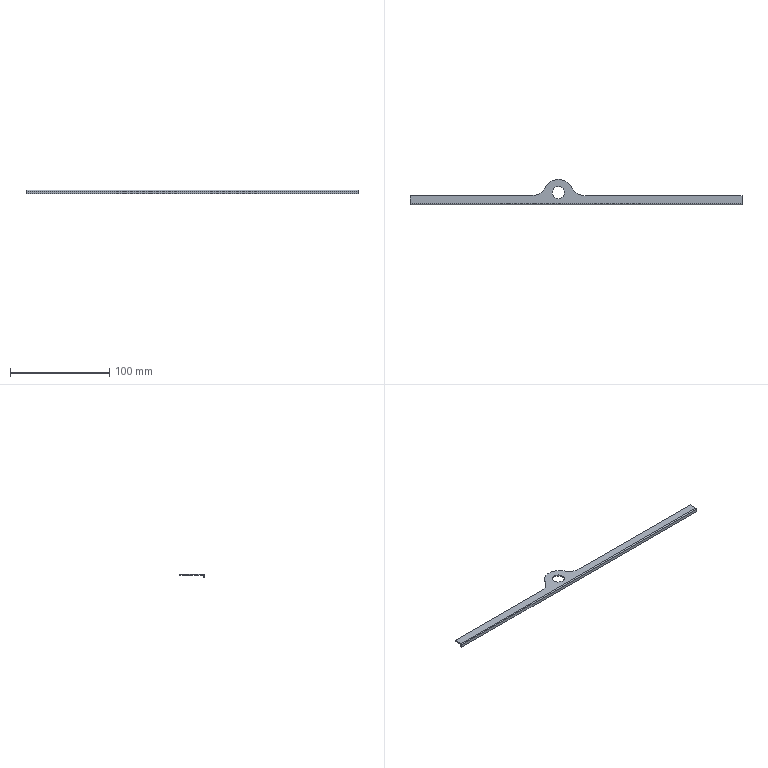Part | STEP file | gslz 2016.10.28-13_id1014_x_t | 1 solid | 14 faces | box 335 x 25.5 x 4 mm | volume 5252 mm3 | plane 9 | cylinder 5 | commonest cylinder face diameters 30 x3 2 x1 12.3 x1
STEP:
#1=CARTESIAN_POINT('',(0.,0.,0.));
#2=DIRECTION('',(0.,0.,1.));
#3=DIRECTION('',(1.,0.,0.));
#4=AXIS2_PLACEMENT_3D('',#1,#2,#3);
#5=CARTESIAN_POINT('',(1374.237,-257.,1.25));
#6=VERTEX_POINT('',#5);
#7=CARTESIAN_POINT('',(1532.655,-257.,1.25));
#8=VERTEX_POINT('',#7);
#9=CARTESIAN_POINT('',(-864.517,-257.,1.25));
#10=DIRECTION('',(1.,0.,0.));
#11=VECTOR('',#10,1.);
#12=LINE('',#9,#11);
#13=CARTESIAN_POINT('',(1375.731,-257.,2.5));
#14=DIRECTION('',(0.,1.,0.));
#15=DIRECTION('',(-1.,0.,0.));
#16=AXIS2_PLACEMENT_3D('',#13,#14,#15);
#17=PLANE('',#16);
#18=CARTESIAN_POINT('',(2240.248,-1.25));
#19=DIRECTION('',(-1.,0.));
#20=VECTOR('',#19,1.);
#21=LINE('',#18,#20);
#22=(GEOMETRIC_REPRESENTATION_CONTEXT(2)PARAMETRIC_REPRESENTATION_CONTEXT()REPRESENTATION_CONTEXT('',''));
#23=DEFINITIONAL_REPRESENTATION('',(#21),#22);
#24=PCURVE('',#17,#23);
#25=CARTESIAN_POINT('',(-864.517,-331.067,1.25));
#26=DIRECTION('',(0.,0.,1.));
#27=DIRECTION('',(-1.,0.,0.));
#28=AXIS2_PLACEMENT_3D('',#25,#26,#27);
#29=PLANE('',#28);
#30=CARTESIAN_POINT('',(0.,-74.067));
#31=DIRECTION('',(-1.,0.));
#32=VECTOR('',#31,1.);
#33=LINE('',#30,#32);
#34=(GEOMETRIC_REPRESENTATION_CONTEXT(2)PARAMETRIC_REPRESENTATION_CONTEXT()REPRESENTATION_CONTEXT('',''));
#35=DEFINITIONAL_REPRESENTATION('',(#33),#34);
#36=PCURVE('',#29,#35);
#37=SURFACE_CURVE('',#12,(#24,#36),.PCURVE_S1.);
#38=EDGE_CURVE('',#6,#8,#37,.T.);
#39=ORIENTED_EDGE('',*,*,#38,.T.);
#40=CARTESIAN_POINT('',(1532.655,-257.,0.));
#41=VERTEX_POINT('',#40);
#42=CARTESIAN_POINT('',(1532.655,-257.,2.5));
#43=DIRECTION('',(0.,0.,1.));
#44=VECTOR('',#43,1.);
#45=LINE('',#42,#44);
#46=CARTESIAN_POINT('',(-156.924,0.));
#47=DIRECTION('',(0.,1.));
#48=VECTOR('',#47,1.);
#49=LINE('',#46,#48);
#50=(GEOMETRIC_REPRESENTATION_CONTEXT(2)PARAMETRIC_REPRESENTATION_CONTEXT()REPRESENTATION_CONTEXT('',''));
#51=DEFINITIONAL_REPRESENTATION('',(#49),#50);
#52=PCURVE('',#17,#51);
#53=CARTESIAN_POINT('',(1532.655,-261.5,-0.75));
#54=DIRECTION('',(1.,0.,0.));
#55=DIRECTION('',(0.,1.,0.));
#56=AXIS2_PLACEMENT_3D('',#53,#54,#55);
#57=PLANE('',#56);
#58=CARTESIAN_POINT('',(4.5,3.25));
#59=DIRECTION('',(0.,1.));
#60=VECTOR('',#59,1.);
#61=LINE('',#58,#60);
#62=(GEOMETRIC_REPRESENTATION_CONTEXT(2)PARAMETRIC_REPRESENTATION_CONTEXT()REPRESENTATION_CONTEXT('',''));
#63=DEFINITIONAL_REPRESENTATION('',(#61),#62);
#64=PCURVE('',#57,#63);
#65=SURFACE_CURVE('',#45,(#52,#64),.PCURVE_S1.);
#66=EDGE_CURVE('',#41,#8,#65,.T.);
#67=ORIENTED_EDGE('',*,*,#66,.F.);
#68=CARTESIAN_POINT('',(1374.237,-257.,0.));
#69=VERTEX_POINT('',#68);
#70=CARTESIAN_POINT('',(1375.731,-257.,0.));
#71=DIRECTION('',(-1.,0.,0.));
#72=VECTOR('',#71,1.);
#73=LINE('',#70,#72);
#74=CARTESIAN_POINT('',(0.,-2.5));
#75=DIRECTION('',(1.,0.));
#76=VECTOR('',#75,1.);
#77=LINE('',#74,#76);
#78=(GEOMETRIC_REPRESENTATION_CONTEXT(2)PARAMETRIC_REPRESENTATION_CONTEXT()REPRESENTATION_CONTEXT('',''));
#79=DEFINITIONAL_REPRESENTATION('',(#77),#78);
#80=PCURVE('',#17,#79);
#81=CARTESIAN_POINT('',(-864.517,-331.067,0.));
#82=DIRECTION('',(0.,0.,1.));
#83=DIRECTION('',(-1.,0.,0.));
#84=AXIS2_PLACEMENT_3D('',#81,#82,#83);
#85=PLANE('',#84);
#86=CARTESIAN_POINT('',(-2240.248,-74.067));
#87=DIRECTION('',(1.,0.));
#88=VECTOR('',#87,1.);
#89=LINE('',#86,#88);
#90=(GEOMETRIC_REPRESENTATION_CONTEXT(2)PARAMETRIC_REPRESENTATION_CONTEXT()REPRESENTATION_CONTEXT('',''));
#91=DEFINITIONAL_REPRESENTATION('',(#89),#90);
#92=PCURVE('',#85,#91);
#93=SURFACE_CURVE('',#73,(#80,#92),.PCURVE_S1.);
#94=EDGE_CURVE('',#41,#69,#93,.T.);
#95=ORIENTED_EDGE('',*,*,#94,.T.);
#96=CARTESIAN_POINT('',(1374.237,-257.,2.5));
#97=DIRECTION('',(0.,0.,1.));
#98=VECTOR('',#97,1.);
#99=LINE('',#96,#98);
#100=CARTESIAN_POINT('',(1.493,0.));
#101=DIRECTION('',(0.,1.));
#102=VECTOR('',#101,1.);
#103=LINE('',#100,#102);
#104=(GEOMETRIC_REPRESENTATION_CONTEXT(2)PARAMETRIC_REPRESENTATION_CONTEXT()REPRESENTATION_CONTEXT('',''));
#105=DEFINITIONAL_REPRESENTATION('',(#103),#104);
#106=PCURVE('',#17,#105);
#107=CARTESIAN_POINT('',(1374.237,-242.,2.5));
#108=DIRECTION('',(0.,0.,-1.));
#109=DIRECTION('',(1.,0.,0.));
#110=AXIS2_PLACEMENT_3D('',#107,#108,#109);
#111=CYLINDRICAL_SURFACE('',#110,15.);
#112=CARTESIAN_POINT('',(1.571,0.));
#113=DIRECTION('',(0.,-1.));
#114=VECTOR('',#113,1.);
#115=LINE('',#112,#114);
#116=(GEOMETRIC_REPRESENTATION_CONTEXT(2)PARAMETRIC_REPRESENTATION_CONTEXT()REPRESENTATION_CONTEXT('',''));
#117=DEFINITIONAL_REPRESENTATION('',(#115),#116);
#118=PCURVE('',#111,#117);
#119=SURFACE_CURVE('',#99,(#106,#118),.PCURVE_S1.);
#120=EDGE_CURVE('',#69,#6,#119,.T.);
#121=ORIENTED_EDGE('',*,*,#120,.T.);
#122=EDGE_LOOP('',(#39,#67,#95,#121));
#123=FACE_BOUND('',#122,.T.);
#124=ADVANCED_FACE('',(#123),#17,.T.);
#125=CARTESIAN_POINT('',(1341.296,-254.,1.25));
#126=VERTEX_POINT('',#125);
#127=CARTESIAN_POINT('',(1347.446,-254.,1.25));
#128=DIRECTION('',(0.,0.,1.));
#129=DIRECTION('',(-1.,0.,0.));
#130=AXIS2_PLACEMENT_3D('',#127,#128,#129);
#131=CIRCLE('',#130,6.15);
#132=CARTESIAN_POINT('',(-2211.964,-77.067));
#133=DIRECTION('',(1.,0.));
#134=AXIS2_PLACEMENT_2D('',#132,#133);
#135=CIRCLE('',#134,6.15);
#136=(GEOMETRIC_REPRESENTATION_CONTEXT(2)PARAMETRIC_REPRESENTATION_CONTEXT()REPRESENTATION_CONTEXT('',''));
#137=DEFINITIONAL_REPRESENTATION('',(#135),#136);
#138=PCURVE('',#29,#137);
#139=CARTESIAN_POINT('',(1347.446,-254.,2.5));
#140=DIRECTION('',(0.,0.,-1.));
#141=DIRECTION('',(1.,0.,0.));
#142=AXIS2_PLACEMENT_3D('',#139,#140,#141);
#143=CYLINDRICAL_SURFACE('',#142,6.15);
#144=CARTESIAN_POINT('',(9.425,1.25));
#145=DIRECTION('',(-1.,0.));
#146=VECTOR('',#145,1.);
#147=LINE('',#144,#146);
#148=(GEOMETRIC_REPRESENTATION_CONTEXT(2)PARAMETRIC_REPRESENTATION_CONTEXT()REPRESENTATION_CONTEXT('',''));
#149=DEFINITIONAL_REPRESENTATION('',(#147),#148);
#150=PCURVE('',#143,#149);
#151=SURFACE_CURVE('',#131,(#138,#150),.PCURVE_S1.);
#152=EDGE_CURVE('',#126,#126,#151,.T.);
#153=ORIENTED_EDGE('',*,*,#152,.F.);
#154=EDGE_LOOP('',(#153));
#155=FACE_BOUND('',#154,.T.);
#156=CARTESIAN_POINT('',(1197.655,-265.,1.25));
#157=VERTEX_POINT('',#156);
#158=CARTESIAN_POINT('',(1532.655,-265.,1.25));
#159=VERTEX_POINT('',#158);
#160=CARTESIAN_POINT('',(1555.25,-265.,1.25));
#161=DIRECTION('',(1.,0.,0.));
#162=VECTOR('',#161,1.);
#163=LINE('',#160,#162);
#164=CARTESIAN_POINT('',(-2419.767,-66.067));
#165=DIRECTION('',(-1.,0.));
#166=VECTOR('',#165,1.);
#167=LINE('',#164,#166);
#168=(GEOMETRIC_REPRESENTATION_CONTEXT(2)PARAMETRIC_REPRESENTATION_CONTEXT()REPRESENTATION_CONTEXT('',''));
#169=DEFINITIONAL_REPRESENTATION('',(#167),#168);
#170=PCURVE('',#29,#169);
#171=CARTESIAN_POINT('',(-864.517,-265.,0.25));
#172=DIRECTION('',(1.,0.,0.));
#173=DIRECTION('',(0.,1.,0.));
#174=AXIS2_PLACEMENT_3D('',#171,#172,#173);
#175=CYLINDRICAL_SURFACE('',#174,1.);
#176=CARTESIAN_POINT('',(1.571,2419.767));
#177=DIRECTION('',(0.,1.));
#178=VECTOR('',#177,1.);
#179=LINE('',#176,#178);
#180=(GEOMETRIC_REPRESENTATION_CONTEXT(2)PARAMETRIC_REPRESENTATION_CONTEXT()REPRESENTATION_CONTEXT('',''));
#181=DEFINITIONAL_REPRESENTATION('',(#179),#180);
#182=PCURVE('',#175,#181);
#183=SURFACE_CURVE('',#163,(#170,#182),.PCURVE_S1.);
#184=EDGE_CURVE('',#157,#159,#183,.T.);
#185=ORIENTED_EDGE('',*,*,#184,.T.);
#186=CARTESIAN_POINT('',(1532.655,319.067,1.25));
#187=DIRECTION('',(0.,1.,0.));
#188=VECTOR('',#187,1.);
#189=LINE('',#186,#188);
#190=CARTESIAN_POINT('',(-2397.172,-650.133));
#191=DIRECTION('',(0.,-1.));
#192=VECTOR('',#191,1.);
#193=LINE('',#190,#192);
#194=(GEOMETRIC_REPRESENTATION_CONTEXT(2)PARAMETRIC_REPRESENTATION_CONTEXT()REPRESENTATION_CONTEXT('',''));
#195=DEFINITIONAL_REPRESENTATION('',(#193),#194);
#196=PCURVE('',#29,#195);
#197=CARTESIAN_POINT('',(580.567,2.));
#198=DIRECTION('',(1.,0.));
#199=VECTOR('',#198,1.);
#200=LINE('',#197,#199);
#201=(GEOMETRIC_REPRESENTATION_CONTEXT(2)PARAMETRIC_REPRESENTATION_CONTEXT()REPRESENTATION_CONTEXT('',''));
#202=DEFINITIONAL_REPRESENTATION('',(#200),#201);
#203=PCURVE('',#57,#202);
#204=SURFACE_CURVE('',#189,(#196,#203),.PCURVE_S1.);
#205=EDGE_CURVE('',#159,#8,#204,.T.);
#206=ORIENTED_EDGE('',*,*,#205,.T.);
#207=ORIENTED_EDGE('',*,*,#38,.F.);
#208=CARTESIAN_POINT('',(1360.842,-248.75,1.25));
#209=VERTEX_POINT('',#208);
#210=CARTESIAN_POINT('',(1374.237,-242.,1.25));
#211=DIRECTION('',(0.,0.,-1.));
#212=DIRECTION('',(-1.,0.,0.));
#213=AXIS2_PLACEMENT_3D('',#210,#211,#212);
#214=CIRCLE('',#213,15.);
#215=CARTESIAN_POINT('',(-2223.754,-89.067));
#216=CARTESIAN_POINT('',(-2223.754,-115.047));
#217=CARTESIAN_POINT('',(-2246.254,-102.057));
#218=CARTESIAN_POINT('',(-2268.754,-89.067));
#219=CARTESIAN_POINT('',(-2246.254,-76.076));
#220=CARTESIAN_POINT('',(-2223.754,-63.086));
#221=CARTESIAN_POINT('',(-2223.754,-89.067));
#222=(BOUNDED_CURVE()B_SPLINE_CURVE(2,(#215,#216,#217,#218,#219,#220,#221),.UNSPECIFIED.,.T.,.F.)B_SPLINE_CURVE_WITH_KNOTS((1,2,2,2,2,1),(-2.094,0.,2.094,4.189,6.283,8.378),.UNSPECIFIED.)CURVE()GEOMETRIC_REPRESENTATION_ITEM()RATIONAL_B_SPLINE_CURVE((1.,0.5,1.,0.5,1.,0.5,1.))REPRESENTATION_ITEM(''));
#223=(GEOMETRIC_REPRESENTATION_CONTEXT(2)PARAMETRIC_REPRESENTATION_CONTEXT()REPRESENTATION_CONTEXT('',''));
#224=DEFINITIONAL_REPRESENTATION('',(#222),#223);
#225=PCURVE('',#29,#224);
#226=CARTESIAN_POINT('',(-3.142,1.25));
#227=DIRECTION('',(1.,0.));
#228=VECTOR('',#227,1.);
#229=LINE('',#226,#228);
#230=(GEOMETRIC_REPRESENTATION_CONTEXT(2)PARAMETRIC_REPRESENTATION_CONTEXT()REPRESENTATION_CONTEXT('',''));
#231=DEFINITIONAL_REPRESENTATION('',(#229),#230);
#232=PCURVE('',#111,#231);
#233=SURFACE_CURVE('',#214,(#225,#232),.PCURVE_S1.);
#234=EDGE_CURVE('',#6,#209,#233,.T.);
#235=ORIENTED_EDGE('',*,*,#234,.T.);
#236=CARTESIAN_POINT('',(1334.051,-248.75,1.25));
#237=VERTEX_POINT('',#236);
#238=CARTESIAN_POINT('',(1347.446,-255.5,1.25));
#239=DIRECTION('',(0.,0.,1.));
#240=DIRECTION('',(-1.,0.,0.));
#241=AXIS2_PLACEMENT_3D('',#238,#239,#240);
#242=CIRCLE('',#241,15.);
#243=CARTESIAN_POINT('',(-2211.964,-75.567));
#244=DIRECTION('',(1.,0.));
#245=AXIS2_PLACEMENT_2D('',#243,#244);
#246=CIRCLE('',#245,15.);
#247=(GEOMETRIC_REPRESENTATION_CONTEXT(2)PARAMETRIC_REPRESENTATION_CONTEXT()REPRESENTATION_CONTEXT('',''));
#248=DEFINITIONAL_REPRESENTATION('',(#246),#247);
#249=PCURVE('',#29,#248);
#250=CARTESIAN_POINT('',(1347.446,-255.5,2.5));
#251=DIRECTION('',(0.,0.,-1.));
#252=DIRECTION('',(1.,0.,0.));
#253=AXIS2_PLACEMENT_3D('',#250,#251,#252);
#254=CYLINDRICAL_SURFACE('',#253,15.);
#255=CARTESIAN_POINT('',(9.425,1.25));
#256=DIRECTION('',(-1.,0.));
#257=VECTOR('',#256,1.);
#258=LINE('',#255,#257);
#259=(GEOMETRIC_REPRESENTATION_CONTEXT(2)PARAMETRIC_REPRESENTATION_CONTEXT()REPRESENTATION_CONTEXT('',''));
#260=DEFINITIONAL_REPRESENTATION('',(#258),#259);
#261=PCURVE('',#254,#260);
#262=SURFACE_CURVE('',#242,(#249,#261),.PCURVE_S1.);
#263=EDGE_CURVE('',#209,#237,#262,.T.);
#264=ORIENTED_EDGE('',*,*,#263,.T.);
#265=CARTESIAN_POINT('',(1320.655,-257.,1.25));
#266=VERTEX_POINT('',#265);
#267=CARTESIAN_POINT('',(1320.655,-242.,1.25));
#268=DIRECTION('',(0.,0.,-1.));
#269=DIRECTION('',(-1.,0.,0.));
#270=AXIS2_PLACEMENT_3D('',#267,#268,#269);
#271=CIRCLE('',#270,15.);
#272=CARTESIAN_POINT('',(-2170.173,-89.067));
#273=CARTESIAN_POINT('',(-2170.173,-115.047));
#274=CARTESIAN_POINT('',(-2192.673,-102.057));
#275=CARTESIAN_POINT('',(-2215.173,-89.067));
#276=CARTESIAN_POINT('',(-2192.673,-76.076));
#277=CARTESIAN_POINT('',(-2170.173,-63.086));
#278=CARTESIAN_POINT('',(-2170.173,-89.067));
#279=(BOUNDED_CURVE()B_SPLINE_CURVE(2,(#272,#273,#274,#275,#276,#277,#278),.UNSPECIFIED.,.T.,.F.)B_SPLINE_CURVE_WITH_KNOTS((1,2,2,2,2,1),(-2.094,0.,2.094,4.189,6.283,8.378),.UNSPECIFIED.)CURVE()GEOMETRIC_REPRESENTATION_ITEM()RATIONAL_B_SPLINE_CURVE((1.,0.5,1.,0.5,1.,0.5,1.))REPRESENTATION_ITEM(''));
#280=(GEOMETRIC_REPRESENTATION_CONTEXT(2)PARAMETRIC_REPRESENTATION_CONTEXT()REPRESENTATION_CONTEXT('',''));
#281=DEFINITIONAL_REPRESENTATION('',(#279),#280);
#282=PCURVE('',#29,#281);
#283=CARTESIAN_POINT('',(1320.655,-242.,2.5));
#284=DIRECTION('',(0.,0.,-1.));
#285=DIRECTION('',(1.,0.,0.));
#286=AXIS2_PLACEMENT_3D('',#283,#284,#285);
#287=CYLINDRICAL_SURFACE('',#286,15.);
#288=CARTESIAN_POINT('',(-3.142,1.25));
#289=DIRECTION('',(1.,0.));
#290=VECTOR('',#289,1.);
#291=LINE('',#288,#290);
#292=(GEOMETRIC_REPRESENTATION_CONTEXT(2)PARAMETRIC_REPRESENTATION_CONTEXT()REPRESENTATION_CONTEXT('',''));
#293=DEFINITIONAL_REPRESENTATION('',(#291),#292);
#294=PCURVE('',#287,#293);
#295=SURFACE_CURVE('',#271,(#282,#294),.PCURVE_S1.);
#296=EDGE_CURVE('',#237,#266,#295,.T.);
#297=ORIENTED_EDGE('',*,*,#296,.T.);
#298=CARTESIAN_POINT('',(1197.655,-257.,1.25));
#299=VERTEX_POINT('',#298);
#300=CARTESIAN_POINT('',(-864.517,-257.,1.25));
#301=DIRECTION('',(1.,0.,0.));
#302=VECTOR('',#301,1.);
#303=LINE('',#300,#302);
#304=CARTESIAN_POINT('',(0.,-74.067));
#305=DIRECTION('',(-1.,0.));
#306=VECTOR('',#305,1.);
#307=LINE('',#304,#306);
#308=(GEOMETRIC_REPRESENTATION_CONTEXT(2)PARAMETRIC_REPRESENTATION_CONTEXT()REPRESENTATION_CONTEXT('',''));
#309=DEFINITIONAL_REPRESENTATION('',(#307),#308);
#310=PCURVE('',#29,#309);
#311=CARTESIAN_POINT('',(1340.291,-257.,0.));
#312=DIRECTION('',(0.,1.,0.));
#313=DIRECTION('',(0.,0.,-1.));
#314=AXIS2_PLACEMENT_3D('',#311,#312,#313);
#315=PLANE('',#314);
#316=CARTESIAN_POINT('',(-1.25,2204.808));
#317=DIRECTION('',(0.,-1.));
#318=VECTOR('',#317,1.);
#319=LINE('',#316,#318);
#320=(GEOMETRIC_REPRESENTATION_CONTEXT(2)PARAMETRIC_REPRESENTATION_CONTEXT()REPRESENTATION_CONTEXT('',''));
#321=DEFINITIONAL_REPRESENTATION('',(#319),#320);
#322=PCURVE('',#315,#321);
#323=SURFACE_CURVE('',#303,(#310,#322),.PCURVE_S1.);
#324=EDGE_CURVE('',#299,#266,#323,.T.);
#325=ORIENTED_EDGE('',*,*,#324,.F.);
#326=CARTESIAN_POINT('',(1197.655,-331.067,1.25));
#327=DIRECTION('',(0.,1.,0.));
#328=VECTOR('',#327,1.);
#329=LINE('',#326,#328);
#330=CARTESIAN_POINT('',(-2062.172,0.));
#331=DIRECTION('',(0.,-1.));
#332=VECTOR('',#331,1.);
#333=LINE('',#330,#332);
#334=(GEOMETRIC_REPRESENTATION_CONTEXT(2)PARAMETRIC_REPRESENTATION_CONTEXT()REPRESENTATION_CONTEXT('',''));
#335=DEFINITIONAL_REPRESENTATION('',(#333),#334);
#336=PCURVE('',#29,#335);
#337=CARTESIAN_POINT('',(1197.655,-261.5,-0.75));
#338=DIRECTION('',(1.,0.,0.));
#339=DIRECTION('',(0.,0.,-1.));
#340=AXIS2_PLACEMENT_3D('',#337,#338,#339);
#341=PLANE('',#340);
#342=CARTESIAN_POINT('',(-2.,-69.567));
#343=DIRECTION('',(0.,1.));
#344=VECTOR('',#343,1.);
#345=LINE('',#342,#344);
#346=(GEOMETRIC_REPRESENTATION_CONTEXT(2)PARAMETRIC_REPRESENTATION_CONTEXT()REPRESENTATION_CONTEXT('',''));
#347=DEFINITIONAL_REPRESENTATION('',(#345),#346);
#348=PCURVE('',#341,#347);
#349=SURFACE_CURVE('',#329,(#336,#348),.PCURVE_S1.);
#350=EDGE_CURVE('',#157,#299,#349,.T.);
#351=ORIENTED_EDGE('',*,*,#350,.F.);
#352=EDGE_LOOP('',(#185,#206,#207,#235,#264,#297,#325,#351));
#353=FACE_BOUND('',#352,.T.);
#354=ADVANCED_FACE('',(#155,#353),#29,.T.);
#355=CARTESIAN_POINT('',(1341.296,-254.,0.));
#356=VERTEX_POINT('',#355);
#357=CARTESIAN_POINT('',(1347.446,-254.,0.));
#358=DIRECTION('',(0.,0.,-1.));
#359=DIRECTION('',(-1.,0.,0.));
#360=AXIS2_PLACEMENT_3D('',#357,#358,#359);
#361=CIRCLE('',#360,6.15);
#362=CARTESIAN_POINT('',(-2205.814,-77.067));
#363=CARTESIAN_POINT('',(-2205.814,-87.719));
#364=CARTESIAN_POINT('',(-2215.039,-82.393));
#365=CARTESIAN_POINT('',(-2224.264,-77.067));
#366=CARTESIAN_POINT('',(-2215.039,-71.741));
#367=CARTESIAN_POINT('',(-2205.814,-66.415));
#368=CARTESIAN_POINT('',(-2205.814,-77.067));
#369=(BOUNDED_CURVE()B_SPLINE_CURVE(2,(#362,#363,#364,#365,#366,#367,#368),.UNSPECIFIED.,.T.,.F.)B_SPLINE_CURVE_WITH_KNOTS((1,2,2,2,2,1),(-2.094,0.,2.094,4.189,6.283,8.378),.UNSPECIFIED.)CURVE()GEOMETRIC_REPRESENTATION_ITEM()RATIONAL_B_SPLINE_CURVE((1.,0.5,1.,0.5,1.,0.5,1.))REPRESENTATION_ITEM(''));
#370=(GEOMETRIC_REPRESENTATION_CONTEXT(2)PARAMETRIC_REPRESENTATION_CONTEXT()REPRESENTATION_CONTEXT('',''));
#371=DEFINITIONAL_REPRESENTATION('',(#369),#370);
#372=PCURVE('',#85,#371);
#373=CARTESIAN_POINT('',(3.142,2.5));
#374=DIRECTION('',(1.,0.));
#375=VECTOR('',#374,1.);
#376=LINE('',#373,#375);
#377=(GEOMETRIC_REPRESENTATION_CONTEXT(2)PARAMETRIC_REPRESENTATION_CONTEXT()REPRESENTATION_CONTEXT('',''));
#378=DEFINITIONAL_REPRESENTATION('',(#376),#377);
#379=PCURVE('',#143,#378);
#380=SURFACE_CURVE('',#361,(#372,#379),.PCURVE_S1.);
#381=EDGE_CURVE('',#356,#356,#380,.T.);
#382=ORIENTED_EDGE('',*,*,#381,.F.);
#383=EDGE_LOOP('',(#382));
#384=FACE_BOUND('',#383,.T.);
#385=ORIENTED_EDGE('',*,*,#94,.F.);
#386=CARTESIAN_POINT('',(1532.655,-264.75,0.));
#387=VERTEX_POINT('',#386);
#388=CARTESIAN_POINT('',(1532.655,319.067,0.));
#389=DIRECTION('',(0.,-1.,0.));
#390=VECTOR('',#389,1.);
#391=LINE('',#388,#390);
#392=CARTESIAN_POINT('',(-2397.172,-650.133));
#393=DIRECTION('',(0.,1.));
#394=VECTOR('',#393,1.);
#395=LINE('',#392,#394);
#396=(GEOMETRIC_REPRESENTATION_CONTEXT(2)PARAMETRIC_REPRESENTATION_CONTEXT()REPRESENTATION_CONTEXT('',''));
#397=DEFINITIONAL_REPRESENTATION('',(#395),#396);
#398=PCURVE('',#85,#397);
#399=CARTESIAN_POINT('',(580.567,0.75));
#400=DIRECTION('',(-1.,0.));
#401=VECTOR('',#400,1.);
#402=LINE('',#399,#401);
#403=(GEOMETRIC_REPRESENTATION_CONTEXT(2)PARAMETRIC_REPRESENTATION_CONTEXT()REPRESENTATION_CONTEXT('',''));
#404=DEFINITIONAL_REPRESENTATION('',(#402),#403);
#405=PCURVE('',#57,#404);
#406=SURFACE_CURVE('',#391,(#398,#405),.PCURVE_S1.);
#407=EDGE_CURVE('',#41,#387,#406,.T.);
#408=ORIENTED_EDGE('',*,*,#407,.T.);
#409=CARTESIAN_POINT('',(1197.655,-264.75,0.));
#410=VERTEX_POINT('',#409);
#411=CARTESIAN_POINT('',(-624.851,-264.75,0.));
#412=DIRECTION('',(1.,0.,0.));
#413=VECTOR('',#412,1.);
#414=LINE('',#411,#413);
#415=CARTESIAN_POINT('',(-239.666,-66.317));
#416=DIRECTION('',(-1.,0.));
#417=VECTOR('',#416,1.);
#418=LINE('',#415,#417);
#419=(GEOMETRIC_REPRESENTATION_CONTEXT(2)PARAMETRIC_REPRESENTATION_CONTEXT()REPRESENTATION_CONTEXT('',''));
#420=DEFINITIONAL_REPRESENTATION('',(#418),#419);
#421=PCURVE('',#85,#420);
#422=CARTESIAN_POINT('',(-624.851,-264.75,-135.834));
#423=DIRECTION('',(0.,-1.,0.));
#424=DIRECTION('',(-1.,0.,0.));
#425=AXIS2_PLACEMENT_3D('',#422,#423,#424);
#426=PLANE('',#425);
#427=CARTESIAN_POINT('',(0.,-135.834));
#428=DIRECTION('',(-1.,0.));
#429=VECTOR('',#428,1.);
#430=LINE('',#427,#429);
#431=(GEOMETRIC_REPRESENTATION_CONTEXT(2)PARAMETRIC_REPRESENTATION_CONTEXT()REPRESENTATION_CONTEXT('',''));
#432=DEFINITIONAL_REPRESENTATION('',(#430),#431);
#433=PCURVE('',#426,#432);
#434=SURFACE_CURVE('',#414,(#421,#433),.PCURVE_S1.);
#435=EDGE_CURVE('',#410,#387,#434,.T.);
#436=ORIENTED_EDGE('',*,*,#435,.F.);
#437=CARTESIAN_POINT('',(1197.655,-257.,0.));
#438=VERTEX_POINT('',#437);
#439=CARTESIAN_POINT('',(1197.655,-331.067,0.));
#440=DIRECTION('',(0.,1.,0.));
#441=VECTOR('',#440,1.);
#442=LINE('',#439,#441);
#443=CARTESIAN_POINT('',(-2062.172,0.));
#444=DIRECTION('',(0.,-1.));
#445=VECTOR('',#444,1.);
#446=LINE('',#443,#445);
#447=(GEOMETRIC_REPRESENTATION_CONTEXT(2)PARAMETRIC_REPRESENTATION_CONTEXT()REPRESENTATION_CONTEXT('',''));
#448=DEFINITIONAL_REPRESENTATION('',(#446),#447);
#449=PCURVE('',#85,#448);
#450=CARTESIAN_POINT('',(-0.75,-69.567));
#451=DIRECTION('',(0.,1.));
#452=VECTOR('',#451,1.);
#453=LINE('',#450,#452);
#454=(GEOMETRIC_REPRESENTATION_CONTEXT(2)PARAMETRIC_REPRESENTATION_CONTEXT()REPRESENTATION_CONTEXT('',''));
#455=DEFINITIONAL_REPRESENTATION('',(#453),#454);
#456=PCURVE('',#341,#455);
#457=SURFACE_CURVE('',#442,(#449,#456),.PCURVE_S1.);
#458=EDGE_CURVE('',#410,#438,#457,.T.);
#459=ORIENTED_EDGE('',*,*,#458,.T.);
#460=CARTESIAN_POINT('',(1320.655,-257.,0.));
#461=VERTEX_POINT('',#460);
#462=CARTESIAN_POINT('',(1340.291,-257.,0.));
#463=DIRECTION('',(-1.,0.,0.));
#464=VECTOR('',#463,1.);
#465=LINE('',#462,#464);
#466=CARTESIAN_POINT('',(-2204.808,-74.067));
#467=DIRECTION('',(1.,0.));
#468=VECTOR('',#467,1.);
#469=LINE('',#466,#468);
#470=(GEOMETRIC_REPRESENTATION_CONTEXT(2)PARAMETRIC_REPRESENTATION_CONTEXT()REPRESENTATION_CONTEXT('',''));
#471=DEFINITIONAL_REPRESENTATION('',(#469),#470);
#472=PCURVE('',#85,#471);
#473=CARTESIAN_POINT('',(0.,0.));
#474=DIRECTION('',(0.,1.));
#475=VECTOR('',#474,1.);
#476=LINE('',#473,#475);
#477=(GEOMETRIC_REPRESENTATION_CONTEXT(2)PARAMETRIC_REPRESENTATION_CONTEXT()REPRESENTATION_CONTEXT('',''));
#478=DEFINITIONAL_REPRESENTATION('',(#476),#477);
#479=PCURVE('',#315,#478);
#480=SURFACE_CURVE('',#465,(#472,#479),.PCURVE_S1.);
#481=EDGE_CURVE('',#461,#438,#480,.T.);
#482=ORIENTED_EDGE('',*,*,#481,.F.);
#483=CARTESIAN_POINT('',(1334.051,-248.75,0.));
#484=VERTEX_POINT('',#483);
#485=CARTESIAN_POINT('',(1320.655,-242.,0.));
#486=DIRECTION('',(0.,0.,1.));
#487=DIRECTION('',(-1.,0.,0.));
#488=AXIS2_PLACEMENT_3D('',#485,#486,#487);
#489=CIRCLE('',#488,15.);
#490=CARTESIAN_POINT('',(-2185.173,-89.067));
#491=DIRECTION('',(1.,0.));
#492=AXIS2_PLACEMENT_2D('',#490,#491);
#493=CIRCLE('',#492,15.);
#494=(GEOMETRIC_REPRESENTATION_CONTEXT(2)PARAMETRIC_REPRESENTATION_CONTEXT()REPRESENTATION_CONTEXT('',''));
#495=DEFINITIONAL_REPRESENTATION('',(#493),#494);
#496=PCURVE('',#85,#495);
#497=CARTESIAN_POINT('',(3.142,2.5));
#498=DIRECTION('',(-1.,0.));
#499=VECTOR('',#498,1.);
#500=LINE('',#497,#499);
#501=(GEOMETRIC_REPRESENTATION_CONTEXT(2)PARAMETRIC_REPRESENTATION_CONTEXT()REPRESENTATION_CONTEXT('',''));
#502=DEFINITIONAL_REPRESENTATION('',(#500),#501);
#503=PCURVE('',#287,#502);
#504=SURFACE_CURVE('',#489,(#496,#503),.PCURVE_S1.);
#505=EDGE_CURVE('',#461,#484,#504,.T.);
#506=ORIENTED_EDGE('',*,*,#505,.T.);
#507=CARTESIAN_POINT('',(1360.842,-248.75,0.));
#508=VERTEX_POINT('',#507);
#509=CARTESIAN_POINT('',(1347.446,-255.5,0.));
#510=DIRECTION('',(0.,0.,-1.));
#511=DIRECTION('',(-1.,0.,0.));
#512=AXIS2_PLACEMENT_3D('',#509,#510,#511);
#513=CIRCLE('',#512,15.);
#514=CARTESIAN_POINT('',(-2196.964,-75.567));
#515=CARTESIAN_POINT('',(-2196.964,-101.547));
#516=CARTESIAN_POINT('',(-2219.464,-88.557));
#517=CARTESIAN_POINT('',(-2241.964,-75.567));
#518=CARTESIAN_POINT('',(-2219.464,-62.576));
#519=CARTESIAN_POINT('',(-2196.964,-49.586));
#520=CARTESIAN_POINT('',(-2196.964,-75.567));
#521=(BOUNDED_CURVE()B_SPLINE_CURVE(2,(#514,#515,#516,#517,#518,#519,#520),.UNSPECIFIED.,.T.,.F.)B_SPLINE_CURVE_WITH_KNOTS((1,2,2,2,2,1),(-2.094,0.,2.094,4.189,6.283,8.378),.UNSPECIFIED.)CURVE()GEOMETRIC_REPRESENTATION_ITEM()RATIONAL_B_SPLINE_CURVE((1.,0.5,1.,0.5,1.,0.5,1.))REPRESENTATION_ITEM(''));
#522=(GEOMETRIC_REPRESENTATION_CONTEXT(2)PARAMETRIC_REPRESENTATION_CONTEXT()REPRESENTATION_CONTEXT('',''));
#523=DEFINITIONAL_REPRESENTATION('',(#521),#522);
#524=PCURVE('',#85,#523);
#525=CARTESIAN_POINT('',(3.142,2.5));
#526=DIRECTION('',(1.,0.));
#527=VECTOR('',#526,1.);
#528=LINE('',#525,#527);
#529=(GEOMETRIC_REPRESENTATION_CONTEXT(2)PARAMETRIC_REPRESENTATION_CONTEXT()REPRESENTATION_CONTEXT('',''));
#530=DEFINITIONAL_REPRESENTATION('',(#528),#529);
#531=PCURVE('',#254,#530);
#532=SURFACE_CURVE('',#513,(#524,#531),.PCURVE_S1.);
#533=EDGE_CURVE('',#484,#508,#532,.T.);
#534=ORIENTED_EDGE('',*,*,#533,.T.);
#535=CARTESIAN_POINT('',(1374.237,-242.,0.));
#536=DIRECTION('',(0.,0.,1.));
#537=DIRECTION('',(-1.,0.,0.));
#538=AXIS2_PLACEMENT_3D('',#535,#536,#537);
#539=CIRCLE('',#538,15.);
#540=CARTESIAN_POINT('',(-2238.754,-89.067));
#541=DIRECTION('',(1.,0.));
#542=AXIS2_PLACEMENT_2D('',#540,#541);
#543=CIRCLE('',#542,15.);
#544=(GEOMETRIC_REPRESENTATION_CONTEXT(2)PARAMETRIC_REPRESENTATION_CONTEXT()REPRESENTATION_CONTEXT('',''));
#545=DEFINITIONAL_REPRESENTATION('',(#543),#544);
#546=PCURVE('',#85,#545);
#547=CARTESIAN_POINT('',(3.142,2.5));
#548=DIRECTION('',(-1.,0.));
#549=VECTOR('',#548,1.);
#550=LINE('',#547,#549);
#551=(GEOMETRIC_REPRESENTATION_CONTEXT(2)PARAMETRIC_REPRESENTATION_CONTEXT()REPRESENTATION_CONTEXT('',''));
#552=DEFINITIONAL_REPRESENTATION('',(#550),#551);
#553=PCURVE('',#111,#552);
#554=SURFACE_CURVE('',#539,(#546,#553),.PCURVE_S1.);
#555=EDGE_CURVE('',#508,#69,#554,.T.);
#556=ORIENTED_EDGE('',*,*,#555,.T.);
#557=EDGE_LOOP('',(#385,#408,#436,#459,#482,#506,#534,#556));
#558=FACE_BOUND('',#557,.T.);
#559=ADVANCED_FACE('',(#384,#558),#85,.F.);
#560=CARTESIAN_POINT('',(1532.655,-264.75,-2.75));
#561=VERTEX_POINT('',#560);
#562=CARTESIAN_POINT('',(1197.655,-264.75,-2.75));
#563=VERTEX_POINT('',#562);
#564=CARTESIAN_POINT('',(2649.074,-264.75,-2.75));
#565=DIRECTION('',(-1.,0.,0.));
#566=VECTOR('',#565,1.);
#567=LINE('',#564,#566);
#568=CARTESIAN_POINT('',(2649.074,-266.,-2.75));
#569=DIRECTION('',(0.,0.,1.));
#570=DIRECTION('',(1.,0.,0.));
#571=AXIS2_PLACEMENT_3D('',#568,#569,#570);
#572=PLANE('',#571);
#573=CARTESIAN_POINT('',(0.,1.25));
#574=DIRECTION('',(-1.,0.));
#575=VECTOR('',#574,1.);
#576=LINE('',#573,#575);
#577=(GEOMETRIC_REPRESENTATION_CONTEXT(2)PARAMETRIC_REPRESENTATION_CONTEXT()REPRESENTATION_CONTEXT('',''));
#578=DEFINITIONAL_REPRESENTATION('',(#576),#577);
#579=PCURVE('',#572,#578);
#580=CARTESIAN_POINT('',(-3273.925,-133.084));
#581=DIRECTION('',(1.,0.));
#582=VECTOR('',#581,1.);
#583=LINE('',#580,#582);
#584=(GEOMETRIC_REPRESENTATION_CONTEXT(2)PARAMETRIC_REPRESENTATION_CONTEXT()REPRESENTATION_CONTEXT('',''));
#585=DEFINITIONAL_REPRESENTATION('',(#583),#584);
#586=PCURVE('',#426,#585);
#587=SURFACE_CURVE('',#567,(#579,#586),.PCURVE_S1.);
#588=EDGE_CURVE('',#561,#563,#587,.T.);
#589=ORIENTED_EDGE('',*,*,#588,.F.);
#590=CARTESIAN_POINT('',(1532.655,-266.,-2.75));
#591=VERTEX_POINT('',#590);
#592=CARTESIAN_POINT('',(1532.655,-266.,-2.75));
#593=DIRECTION('',(0.,1.,0.));
#594=VECTOR('',#593,1.);
#595=LINE('',#592,#594);
#596=CARTESIAN_POINT('',(-1116.419,0.));
#597=DIRECTION('',(0.,1.));
#598=VECTOR('',#597,1.);
#599=LINE('',#596,#598);
#600=(GEOMETRIC_REPRESENTATION_CONTEXT(2)PARAMETRIC_REPRESENTATION_CONTEXT()REPRESENTATION_CONTEXT('',''));
#601=DEFINITIONAL_REPRESENTATION('',(#599),#600);
#602=PCURVE('',#572,#601);
#603=CARTESIAN_POINT('',(-4.5,-2.));
#604=DIRECTION('',(1.,0.));
#605=VECTOR('',#604,1.);
#606=LINE('',#603,#605);
#607=(GEOMETRIC_REPRESENTATION_CONTEXT(2)PARAMETRIC_REPRESENTATION_CONTEXT()REPRESENTATION_CONTEXT('',''));
#608=DEFINITIONAL_REPRESENTATION('',(#606),#607);
#609=PCURVE('',#57,#608);
#610=SURFACE_CURVE('',#595,(#602,#609),.PCURVE_S1.);
#611=EDGE_CURVE('',#591,#561,#610,.T.);
#612=ORIENTED_EDGE('',*,*,#611,.F.);
#613=CARTESIAN_POINT('',(1197.655,-266.,-2.75));
#614=VERTEX_POINT('',#613);
#615=CARTESIAN_POINT('',(2649.074,-266.,-2.75));
#616=DIRECTION('',(-1.,0.,0.));
#617=VECTOR('',#616,1.);
#618=LINE('',#615,#617);
#619=CARTESIAN_POINT('',(0.,0.));
#620=DIRECTION('',(-1.,0.));
#621=VECTOR('',#620,1.);
#622=LINE('',#619,#621);
#623=(GEOMETRIC_REPRESENTATION_CONTEXT(2)PARAMETRIC_REPRESENTATION_CONTEXT()REPRESENTATION_CONTEXT('',''));
#624=DEFINITIONAL_REPRESENTATION('',(#622),#623);
#625=PCURVE('',#572,#624);
#626=CARTESIAN_POINT('',(1387.649,-266.,0.625));
#627=DIRECTION('',(0.,-1.,0.));
#628=DIRECTION('',(-1.,0.,0.));
#629=AXIS2_PLACEMENT_3D('',#626,#627,#628);
#630=PLANE('',#629);
#631=CARTESIAN_POINT('',(-1261.425,3.375));
#632=DIRECTION('',(1.,0.));
#633=VECTOR('',#632,1.);
#634=LINE('',#631,#633);
#635=(GEOMETRIC_REPRESENTATION_CONTEXT(2)PARAMETRIC_REPRESENTATION_CONTEXT()REPRESENTATION_CONTEXT('',''));
#636=DEFINITIONAL_REPRESENTATION('',(#634),#635);
#637=PCURVE('',#630,#636);
#638=SURFACE_CURVE('',#618,(#625,#637),.PCURVE_S1.);
#639=EDGE_CURVE('',#591,#614,#638,.T.);
#640=ORIENTED_EDGE('',*,*,#639,.T.);
#641=CARTESIAN_POINT('',(1197.655,-266.,-2.75));
#642=DIRECTION('',(0.,-1.,0.));
#643=VECTOR('',#642,1.);
#644=LINE('',#641,#643);
#645=CARTESIAN_POINT('',(-1451.419,0.));
#646=DIRECTION('',(0.,-1.));
#647=VECTOR('',#646,1.);
#648=LINE('',#645,#647);
#649=(GEOMETRIC_REPRESENTATION_CONTEXT(2)PARAMETRIC_REPRESENTATION_CONTEXT()REPRESENTATION_CONTEXT('',''));
#650=DEFINITIONAL_REPRESENTATION('',(#648),#649);
#651=PCURVE('',#572,#650);
#652=CARTESIAN_POINT('',(2.,-4.5));
#653=DIRECTION('',(0.,-1.));
#654=VECTOR('',#653,1.);
#655=LINE('',#652,#654);
#656=(GEOMETRIC_REPRESENTATION_CONTEXT(2)PARAMETRIC_REPRESENTATION_CONTEXT()REPRESENTATION_CONTEXT('',''));
#657=DEFINITIONAL_REPRESENTATION('',(#655),#656);
#658=PCURVE('',#341,#657);
#659=SURFACE_CURVE('',#644,(#651,#658),.PCURVE_S1.);
#660=EDGE_CURVE('',#563,#614,#659,.T.);
#661=ORIENTED_EDGE('',*,*,#660,.F.);
#662=EDGE_LOOP('',(#589,#612,#640,#661));
#663=FACE_BOUND('',#662,.T.);
#664=ADVANCED_FACE('',(#663),#572,.F.);
#665=ORIENTED_EDGE('',*,*,#639,.F.);
#666=CARTESIAN_POINT('',(1532.655,-266.,0.25));
#667=VERTEX_POINT('',#666);
#668=CARTESIAN_POINT('',(1532.655,-266.,0.625));
#669=DIRECTION('',(0.,0.,-1.));
#670=VECTOR('',#669,1.);
#671=LINE('',#668,#670);
#672=CARTESIAN_POINT('',(-145.006,0.));
#673=DIRECTION('',(0.,1.));
#674=VECTOR('',#673,1.);
#675=LINE('',#672,#674);
#676=(GEOMETRIC_REPRESENTATION_CONTEXT(2)PARAMETRIC_REPRESENTATION_CONTEXT()REPRESENTATION_CONTEXT('',''));
#677=DEFINITIONAL_REPRESENTATION('',(#675),#676);
#678=PCURVE('',#630,#677);
#679=CARTESIAN_POINT('',(-4.5,1.375));
#680=DIRECTION('',(0.,-1.));
#681=VECTOR('',#680,1.);
#682=LINE('',#679,#681);
#683=(GEOMETRIC_REPRESENTATION_CONTEXT(2)PARAMETRIC_REPRESENTATION_CONTEXT()REPRESENTATION_CONTEXT('',''));
#684=DEFINITIONAL_REPRESENTATION('',(#682),#683);
#685=PCURVE('',#57,#684);
#686=SURFACE_CURVE('',#671,(#678,#685),.PCURVE_S1.);
#687=EDGE_CURVE('',#667,#591,#686,.T.);
#688=ORIENTED_EDGE('',*,*,#687,.F.);
#689=CARTESIAN_POINT('',(1197.655,-266.,0.25));
#690=VERTEX_POINT('',#689);
#691=CARTESIAN_POINT('',(1215.149,-266.,0.25));
#692=DIRECTION('',(-1.,0.,0.));
#693=VECTOR('',#692,1.);
#694=LINE('',#691,#693);
#695=CARTESIAN_POINT('',(172.5,0.375));
#696=DIRECTION('',(1.,0.));
#697=VECTOR('',#696,1.);
#698=LINE('',#695,#697);
#699=(GEOMETRIC_REPRESENTATION_CONTEXT(2)PARAMETRIC_REPRESENTATION_CONTEXT()REPRESENTATION_CONTEXT('',''));
#700=DEFINITIONAL_REPRESENTATION('',(#698),#699);
#701=PCURVE('',#630,#700);
#702=CARTESIAN_POINT('',(3.142,2079.666));
#703=DIRECTION('',(0.,-1.));
#704=VECTOR('',#703,1.);
#705=LINE('',#702,#704);
#706=(GEOMETRIC_REPRESENTATION_CONTEXT(2)PARAMETRIC_REPRESENTATION_CONTEXT()REPRESENTATION_CONTEXT('',''));
#707=DEFINITIONAL_REPRESENTATION('',(#705),#706);
#708=PCURVE('',#175,#707);
#709=SURFACE_CURVE('',#694,(#701,#708),.PCURVE_S1.);
#710=EDGE_CURVE('',#667,#690,#709,.T.);
#711=ORIENTED_EDGE('',*,*,#710,.T.);
#712=CARTESIAN_POINT('',(1197.655,-266.,0.625));
#713=DIRECTION('',(0.,0.,-1.));
#714=VECTOR('',#713,1.);
#715=LINE('',#712,#714);
#716=CARTESIAN_POINT('',(189.994,0.));
#717=DIRECTION('',(0.,1.));
#718=VECTOR('',#717,1.);
#719=LINE('',#716,#718);
#720=(GEOMETRIC_REPRESENTATION_CONTEXT(2)PARAMETRIC_REPRESENTATION_CONTEXT()REPRESENTATION_CONTEXT('',''));
#721=DEFINITIONAL_REPRESENTATION('',(#719),#720);
#722=PCURVE('',#630,#721);
#723=CARTESIAN_POINT('',(-1.375,-4.5));
#724=DIRECTION('',(1.,0.));
#725=VECTOR('',#724,1.);
#726=LINE('',#723,#725);
#727=(GEOMETRIC_REPRESENTATION_CONTEXT(2)PARAMETRIC_REPRESENTATION_CONTEXT()REPRESENTATION_CONTEXT('',''));
#728=DEFINITIONAL_REPRESENTATION('',(#726),#727);
#729=PCURVE('',#341,#728);
#730=SURFACE_CURVE('',#715,(#722,#729),.PCURVE_S1.);
#731=EDGE_CURVE('',#690,#614,#730,.T.);
#732=ORIENTED_EDGE('',*,*,#731,.T.);
#733=EDGE_LOOP('',(#665,#688,#711,#732));
#734=FACE_BOUND('',#733,.T.);
#735=ADVANCED_FACE('',(#734),#630,.T.);
#736=ORIENTED_EDGE('',*,*,#435,.T.);
#737=CARTESIAN_POINT('',(1532.655,-264.75,-135.834));
#738=DIRECTION('',(0.,0.,-1.));
#739=VECTOR('',#738,1.);
#740=LINE('',#737,#739);
#741=CARTESIAN_POINT('',(-2157.506,0.));
#742=DIRECTION('',(0.,1.));
#743=VECTOR('',#742,1.);
#744=LINE('',#741,#743);
#745=(GEOMETRIC_REPRESENTATION_CONTEXT(2)PARAMETRIC_REPRESENTATION_CONTEXT()REPRESENTATION_CONTEXT('',''));
#746=DEFINITIONAL_REPRESENTATION('',(#744),#745);
#747=PCURVE('',#426,#746);
#748=CARTESIAN_POINT('',(-3.25,-135.084));
#749=DIRECTION('',(0.,-1.));
#750=VECTOR('',#749,1.);
#751=LINE('',#748,#750);
#752=(GEOMETRIC_REPRESENTATION_CONTEXT(2)PARAMETRIC_REPRESENTATION_CONTEXT()REPRESENTATION_CONTEXT('',''));
#753=DEFINITIONAL_REPRESENTATION('',(#751),#752);
#754=PCURVE('',#57,#753);
#755=SURFACE_CURVE('',#740,(#747,#754),.PCURVE_S1.);
#756=EDGE_CURVE('',#387,#561,#755,.T.);
#757=ORIENTED_EDGE('',*,*,#756,.T.);
#758=ORIENTED_EDGE('',*,*,#588,.T.);
#759=CARTESIAN_POINT('',(1197.655,-264.75,-135.834));
#760=DIRECTION('',(0.,0.,-1.));
#761=VECTOR('',#760,1.);
#762=LINE('',#759,#761);
#763=CARTESIAN_POINT('',(-1822.506,0.));
#764=DIRECTION('',(0.,1.));
#765=VECTOR('',#764,1.);
#766=LINE('',#763,#765);
#767=(GEOMETRIC_REPRESENTATION_CONTEXT(2)PARAMETRIC_REPRESENTATION_CONTEXT()REPRESENTATION_CONTEXT('',''));
#768=DEFINITIONAL_REPRESENTATION('',(#766),#767);
#769=PCURVE('',#426,#768);
#770=CARTESIAN_POINT('',(135.084,-3.25));
#771=DIRECTION('',(1.,0.));
#772=VECTOR('',#771,1.);
#773=LINE('',#770,#772);
#774=(GEOMETRIC_REPRESENTATION_CONTEXT(2)PARAMETRIC_REPRESENTATION_CONTEXT()REPRESENTATION_CONTEXT('',''));
#775=DEFINITIONAL_REPRESENTATION('',(#773),#774);
#776=PCURVE('',#341,#775);
#777=SURFACE_CURVE('',#762,(#769,#776),.PCURVE_S1.);
#778=EDGE_CURVE('',#410,#563,#777,.T.);
#779=ORIENTED_EDGE('',*,*,#778,.F.);
#780=EDGE_LOOP('',(#736,#757,#758,#779));
#781=FACE_BOUND('',#780,.T.);
#782=ADVANCED_FACE('',(#781),#426,.F.);
#783=ORIENTED_EDGE('',*,*,#710,.F.);
#784=CARTESIAN_POINT('',(1532.655,-265.,0.25));
#785=DIRECTION('',(-1.,0.,0.));
#786=DIRECTION('',(0.,1.,0.));
#787=AXIS2_PLACEMENT_3D('',#784,#785,#786);
#788=CIRCLE('',#787,1.);
#789=CARTESIAN_POINT('',(6.283,2397.172));
#790=DIRECTION('',(-1.,0.));
#791=VECTOR('',#790,1.);
#792=LINE('',#789,#791);
#793=(GEOMETRIC_REPRESENTATION_CONTEXT(2)PARAMETRIC_REPRESENTATION_CONTEXT()REPRESENTATION_CONTEXT('',''));
#794=DEFINITIONAL_REPRESENTATION('',(#792),#793);
#795=PCURVE('',#175,#794);
#796=CARTESIAN_POINT('',(-2.5,1.));
#797=CARTESIAN_POINT('',(-2.5,-0.7321));
#798=CARTESIAN_POINT('',(-4.,0.134));
#799=CARTESIAN_POINT('',(-5.5,1.));
#800=CARTESIAN_POINT('',(-4.,1.866));
#801=CARTESIAN_POINT('',(-2.5,2.732));
#802=CARTESIAN_POINT('',(-2.5,1.));
#803=(BOUNDED_CURVE()B_SPLINE_CURVE(2,(#796,#797,#798,#799,#800,#801,#802),.UNSPECIFIED.,.T.,.F.)B_SPLINE_CURVE_WITH_KNOTS((1,2,2,2,2,1),(-2.094,0.,2.094,4.189,6.283,8.378),.UNSPECIFIED.)CURVE()GEOMETRIC_REPRESENTATION_ITEM()RATIONAL_B_SPLINE_CURVE((1.,0.5,1.,0.5,1.,0.5,1.))REPRESENTATION_ITEM(''));
#804=(GEOMETRIC_REPRESENTATION_CONTEXT(2)PARAMETRIC_REPRESENTATION_CONTEXT()REPRESENTATION_CONTEXT('',''));
#805=DEFINITIONAL_REPRESENTATION('',(#803),#804);
#806=PCURVE('',#57,#805);
#807=SURFACE_CURVE('',#788,(#795,#806),.PCURVE_S1.);
#808=EDGE_CURVE('',#667,#159,#807,.T.);
#809=ORIENTED_EDGE('',*,*,#808,.T.);
#810=ORIENTED_EDGE('',*,*,#184,.F.);
#811=CARTESIAN_POINT('',(1197.655,-265.,0.25));
#812=DIRECTION('',(-1.,0.,0.));
#813=DIRECTION('',(0.,0.,-1.));
#814=AXIS2_PLACEMENT_3D('',#811,#812,#813);
#815=CIRCLE('',#814,1.);
#816=CARTESIAN_POINT('',(4.712,2062.172));
#817=DIRECTION('',(-1.,0.));
#818=VECTOR('',#817,1.);
#819=LINE('',#816,#818);
#820=(GEOMETRIC_REPRESENTATION_CONTEXT(2)PARAMETRIC_REPRESENTATION_CONTEXT()REPRESENTATION_CONTEXT('',''));
#821=DEFINITIONAL_REPRESENTATION('',(#819),#820);
#822=PCURVE('',#175,#821);
#823=CARTESIAN_POINT('',(0.,-3.5));
#824=CARTESIAN_POINT('',(0.,-5.232));
#825=CARTESIAN_POINT('',(-1.5,-4.366));
#826=CARTESIAN_POINT('',(-3.,-3.5));
#827=CARTESIAN_POINT('',(-1.5,-2.634));
#828=CARTESIAN_POINT('',(0.,-1.768));
#829=CARTESIAN_POINT('',(0.,-3.5));
#830=(BOUNDED_CURVE()B_SPLINE_CURVE(2,(#823,#824,#825,#826,#827,#828,#829),.UNSPECIFIED.,.T.,.F.)B_SPLINE_CURVE_WITH_KNOTS((1,2,2,2,2,1),(-2.094,0.,2.094,4.189,6.283,8.378),.UNSPECIFIED.)CURVE()GEOMETRIC_REPRESENTATION_ITEM()RATIONAL_B_SPLINE_CURVE((1.,0.5,1.,0.5,1.,0.5,1.))REPRESENTATION_ITEM(''));
#831=(GEOMETRIC_REPRESENTATION_CONTEXT(2)PARAMETRIC_REPRESENTATION_CONTEXT()REPRESENTATION_CONTEXT('',''));
#832=DEFINITIONAL_REPRESENTATION('',(#830),#831);
#833=PCURVE('',#341,#832);
#834=SURFACE_CURVE('',#815,(#822,#833),.PCURVE_S1.);
#835=EDGE_CURVE('',#690,#157,#834,.T.);
#836=ORIENTED_EDGE('',*,*,#835,.F.);
#837=EDGE_LOOP('',(#783,#809,#810,#836));
#838=FACE_BOUND('',#837,.T.);
#839=ADVANCED_FACE('',(#838),#175,.T.);
#840=ORIENTED_EDGE('',*,*,#152,.F.);
#841=CARTESIAN_POINT('',(1341.296,-254.,1.25));
#842=CARTESIAN_POINT('',(1341.296,-254.,0.));
#843=B_SPLINE_CURVE_WITH_KNOTS('',1,(#841,#842),.UNSPECIFIED.,.F.,.F.,(2,2),(1.25,2.5),.PIECEWISE_BEZIER_KNOTS.);
#844=CARTESIAN_POINT('',(9.425,0.));
#845=DIRECTION('',(0.,1.));
#846=VECTOR('',#845,1.);
#847=LINE('',#844,#846);
#848=(GEOMETRIC_REPRESENTATION_CONTEXT(2)PARAMETRIC_REPRESENTATION_CONTEXT()REPRESENTATION_CONTEXT('',''));
#849=DEFINITIONAL_REPRESENTATION('',(#847),#848);
#850=PCURVE('',#143,#849);
#851=CARTESIAN_POINT('',(3.142,0.));
#852=DIRECTION('',(0.,1.));
#853=VECTOR('',#852,1.);
#854=LINE('',#851,#853);
#855=(GEOMETRIC_REPRESENTATION_CONTEXT(2)PARAMETRIC_REPRESENTATION_CONTEXT()REPRESENTATION_CONTEXT('',''));
#856=DEFINITIONAL_REPRESENTATION('',(#854),#855);
#857=PCURVE('',#143,#856);
#858=SEAM_CURVE('',#843,(#850,#857),.PCURVE_S1.);
#859=EDGE_CURVE('',#126,#356,#858,.T.);
#860=ORIENTED_EDGE('',*,*,#859,.T.);
#861=ORIENTED_EDGE('',*,*,#381,.F.);
#862=ORIENTED_EDGE('',*,*,#859,.F.);
#863=EDGE_LOOP('',(#840,#860,#861,#862));
#864=FACE_BOUND('',#863,.F.);
#865=ADVANCED_FACE('',(#864),#143,.F.);
#866=ORIENTED_EDGE('',*,*,#481,.T.);
#867=CARTESIAN_POINT('',(1197.655,-257.,2.5));
#868=DIRECTION('',(0.,0.,1.));
#869=VECTOR('',#868,1.);
#870=LINE('',#867,#869);
#871=CARTESIAN_POINT('',(-2.5,142.636));
#872=DIRECTION('',(-1.,0.));
#873=VECTOR('',#872,1.);
#874=LINE('',#871,#873);
#875=(GEOMETRIC_REPRESENTATION_CONTEXT(2)PARAMETRIC_REPRESENTATION_CONTEXT()REPRESENTATION_CONTEXT('',''));
#876=DEFINITIONAL_REPRESENTATION('',(#874),#875);
#877=PCURVE('',#315,#876);
#878=CARTESIAN_POINT('',(-3.25,4.5));
#879=DIRECTION('',(-1.,0.));
#880=VECTOR('',#879,1.);
#881=LINE('',#878,#880);
#882=(GEOMETRIC_REPRESENTATION_CONTEXT(2)PARAMETRIC_REPRESENTATION_CONTEXT()REPRESENTATION_CONTEXT('',''));
#883=DEFINITIONAL_REPRESENTATION('',(#881),#882);
#884=PCURVE('',#341,#883);
#885=SURFACE_CURVE('',#870,(#877,#884),.PCURVE_S1.);
#886=EDGE_CURVE('',#438,#299,#885,.T.);
#887=ORIENTED_EDGE('',*,*,#886,.T.);
#888=ORIENTED_EDGE('',*,*,#324,.T.);
#889=CARTESIAN_POINT('',(1320.655,-257.,2.5));
#890=DIRECTION('',(0.,0.,1.));
#891=VECTOR('',#890,1.);
#892=LINE('',#889,#891);
#893=CARTESIAN_POINT('',(-2.5,19.635));
#894=DIRECTION('',(-1.,0.));
#895=VECTOR('',#894,1.);
#896=LINE('',#893,#895);
#897=(GEOMETRIC_REPRESENTATION_CONTEXT(2)PARAMETRIC_REPRESENTATION_CONTEXT()REPRESENTATION_CONTEXT('',''));
#898=DEFINITIONAL_REPRESENTATION('',(#896),#897);
#899=PCURVE('',#315,#898);
#900=CARTESIAN_POINT('',(1.571,0.));
#901=DIRECTION('',(0.,-1.));
#902=VECTOR('',#901,1.);
#903=LINE('',#900,#902);
#904=(GEOMETRIC_REPRESENTATION_CONTEXT(2)PARAMETRIC_REPRESENTATION_CONTEXT()REPRESENTATION_CONTEXT('',''));
#905=DEFINITIONAL_REPRESENTATION('',(#903),#904);
#906=PCURVE('',#287,#905);
#907=SURFACE_CURVE('',#892,(#899,#906),.PCURVE_S1.);
#908=EDGE_CURVE('',#461,#266,#907,.T.);
#909=ORIENTED_EDGE('',*,*,#908,.F.);
#910=EDGE_LOOP('',(#866,#887,#888,#909));
#911=FACE_BOUND('',#910,.T.);
#912=ADVANCED_FACE('',(#911),#315,.T.);
#913=ORIENTED_EDGE('',*,*,#533,.F.);
#914=CARTESIAN_POINT('',(1334.051,-248.75,0.625));
#915=DIRECTION('',(0.,0.,1.));
#916=VECTOR('',#915,1.);
#917=LINE('',#914,#916);
#918=CARTESIAN_POINT('',(3.608,1.875));
#919=DIRECTION('',(0.,-1.));
#920=VECTOR('',#919,1.);
#921=LINE('',#918,#920);
#922=(GEOMETRIC_REPRESENTATION_CONTEXT(2)PARAMETRIC_REPRESENTATION_CONTEXT()REPRESENTATION_CONTEXT('',''));
#923=DEFINITIONAL_REPRESENTATION('',(#921),#922);
#924=PCURVE('',#254,#923);
#925=CARTESIAN_POINT('',(0.4668,1.875));
#926=DIRECTION('',(0.,-1.));
#927=VECTOR('',#926,1.);
#928=LINE('',#925,#927);
#929=(GEOMETRIC_REPRESENTATION_CONTEXT(2)PARAMETRIC_REPRESENTATION_CONTEXT()REPRESENTATION_CONTEXT('',''));
#930=DEFINITIONAL_REPRESENTATION('',(#928),#929);
#931=PCURVE('',#287,#930);
#932=SURFACE_CURVE('',#917,(#924,#931),.PCURVE_S1.);
#933=EDGE_CURVE('',#484,#237,#932,.T.);
#934=ORIENTED_EDGE('',*,*,#933,.T.);
#935=ORIENTED_EDGE('',*,*,#263,.F.);
#936=CARTESIAN_POINT('',(1360.842,-248.75,0.625));
#937=DIRECTION('',(0.,0.,1.));
#938=VECTOR('',#937,1.);
#939=LINE('',#936,#938);
#940=CARTESIAN_POINT('',(5.816,1.875));
#941=DIRECTION('',(0.,-1.));
#942=VECTOR('',#941,1.);
#943=LINE('',#940,#942);
#944=(GEOMETRIC_REPRESENTATION_CONTEXT(2)PARAMETRIC_REPRESENTATION_CONTEXT()REPRESENTATION_CONTEXT('',''));
#945=DEFINITIONAL_REPRESENTATION('',(#943),#944);
#946=PCURVE('',#254,#945);
#947=CARTESIAN_POINT('',(2.675,1.875));
#948=DIRECTION('',(0.,-1.));
#949=VECTOR('',#948,1.);
#950=LINE('',#947,#949);
#951=(GEOMETRIC_REPRESENTATION_CONTEXT(2)PARAMETRIC_REPRESENTATION_CONTEXT()REPRESENTATION_CONTEXT('',''));
#952=DEFINITIONAL_REPRESENTATION('',(#950),#951);
#953=PCURVE('',#111,#952);
#954=SURFACE_CURVE('',#939,(#946,#953),.PCURVE_S1.);
#955=EDGE_CURVE('',#508,#209,#954,.T.);
#956=ORIENTED_EDGE('',*,*,#955,.F.);
#957=EDGE_LOOP('',(#913,#934,#935,#956));
#958=FACE_BOUND('',#957,.T.);
#959=ADVANCED_FACE('',(#958),#254,.T.);
#960=ORIENTED_EDGE('',*,*,#296,.T.);
#961=ORIENTED_EDGE('',*,*,#908,.F.);
#962=ORIENTED_EDGE('',*,*,#505,.T.);
#963=ORIENTED_EDGE('',*,*,#933,.T.);
#964=EDGE_LOOP('',(#960,#961,#962,#963));
#965=FACE_BOUND('',#964,.F.);
#966=ADVANCED_FACE('',(#965),#287,.F.);
#967=ORIENTED_EDGE('',*,*,#234,.T.);
#968=ORIENTED_EDGE('',*,*,#955,.F.);
#969=ORIENTED_EDGE('',*,*,#555,.T.);
#970=ORIENTED_EDGE('',*,*,#120,.T.);
#971=EDGE_LOOP('',(#967,#968,#969,#970));
#972=FACE_BOUND('',#971,.F.);
#973=ADVANCED_FACE('',(#972),#111,.F.);
#974=ORIENTED_EDGE('',*,*,#687,.T.);
#975=ORIENTED_EDGE('',*,*,#611,.T.);
#976=ORIENTED_EDGE('',*,*,#756,.F.);
#977=ORIENTED_EDGE('',*,*,#407,.F.);
#978=ORIENTED_EDGE('',*,*,#66,.T.);
#979=ORIENTED_EDGE('',*,*,#205,.F.);
#980=ORIENTED_EDGE('',*,*,#808,.F.);
#981=EDGE_LOOP('',(#974,#975,#976,#977,#978,#979,#980));
#982=FACE_BOUND('',#981,.T.);
#983=ADVANCED_FACE('',(#982),#57,.T.);
#984=ORIENTED_EDGE('',*,*,#778,.T.);
#985=ORIENTED_EDGE('',*,*,#660,.T.);
#986=ORIENTED_EDGE('',*,*,#731,.F.);
#987=ORIENTED_EDGE('',*,*,#835,.T.);
#988=ORIENTED_EDGE('',*,*,#350,.T.);
#989=ORIENTED_EDGE('',*,*,#886,.F.);
#990=ORIENTED_EDGE('',*,*,#458,.F.);
#991=EDGE_LOOP('',(#984,#985,#986,#987,#988,#989,#990));
#992=FACE_BOUND('',#991,.T.);
#993=ADVANCED_FACE('',(#992),#341,.F.);
#994=CLOSED_SHELL('',(#124,#354,#559,#664,#735,#782,#839,#865,#912,#959,#966,#973,#983,#993));
#995=MANIFOLD_SOLID_BREP('',#994);
#996=(LENGTH_UNIT()NAMED_UNIT(*)SI_UNIT(.MILLI.,.METRE.));
#997=UNCERTAINTY_MEASURE_WITH_UNIT(LENGTH_MEASURE(0.000001),#996,'','');
#998=(NAMED_UNIT(*)PLANE_ANGLE_UNIT()SI_UNIT($,.RADIAN.));
#999=(NAMED_UNIT(*)SI_UNIT($,.STERADIAN.)SOLID_ANGLE_UNIT());
#1000=(GEOMETRIC_REPRESENTATION_CONTEXT(3)GLOBAL_UNCERTAINTY_ASSIGNED_CONTEXT((#997))GLOBAL_UNIT_ASSIGNED_CONTEXT((#996,#998,#999))REPRESENTATION_CONTEXT('',''));
#1001=ADVANCED_BREP_SHAPE_REPRESENTATION('',(#4,#995),#1000);